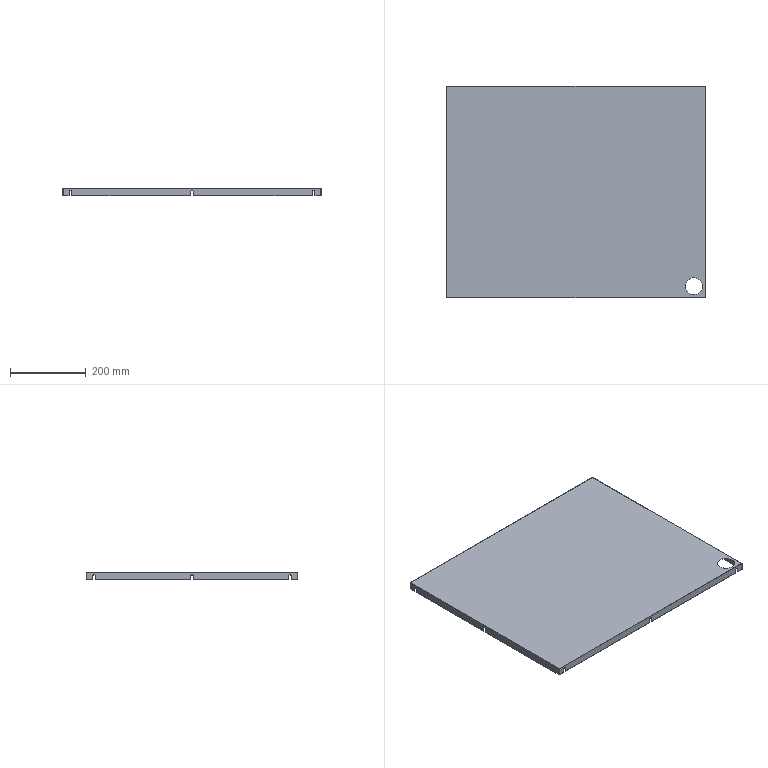Part | STEP file | PN_0008 | 1 solid | 66 faces | box 683 x 558 x 20 mm | volume 425535 mm3 | plane 46 | cylinder 20 | commonest cylinder face diameters 7 x18 45 x2